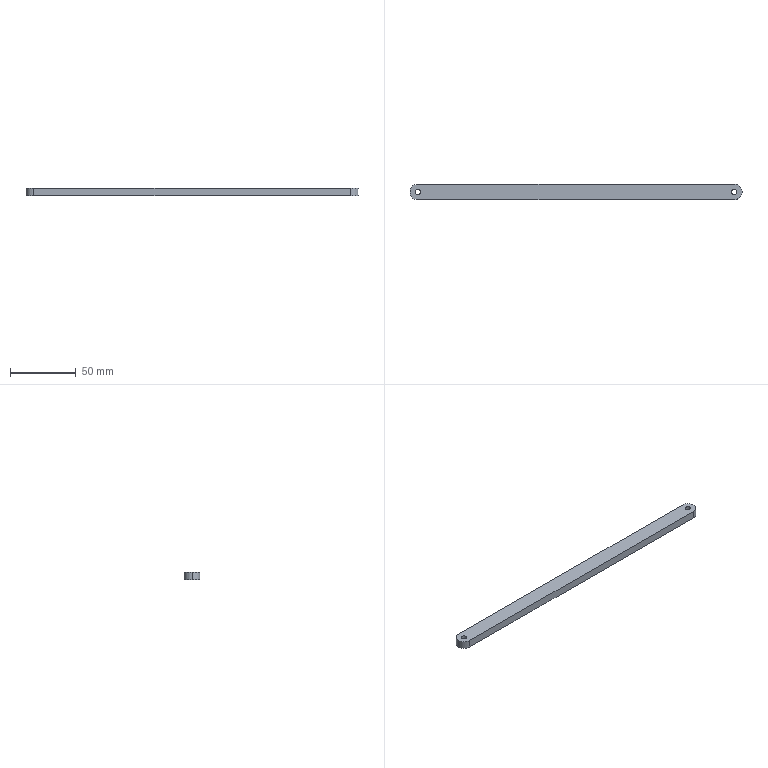Part | SolidWorks | features Extrusion 1 | 1 solid | 11 faces | box 252 x 12 x 6 mm | volume 17808 mm3 | cylinder 7 | plane 4 | commonest cylinder face diameters 4 x4 12 x3
STEP:
#1=CARTESIAN_POINT('',(118.265,1.191,6.));
#2=VERTEX_POINT('',#1);
#3=CARTESIAN_POINT('',(122.265,1.191,6.));
#4=VERTEX_POINT('',#3);
#5=CARTESIAN_POINT('',(120.265,1.191,6.));
#6=DIRECTION('',(0.,0.,1.));
#7=DIRECTION('',(1.,0.,0.));
#8=AXIS2_PLACEMENT_3D('',#5,#6,#7);
#9=CIRCLE('',#8,2.);
#10=EDGE_CURVE('',#2,#4,#9,.T.);
#11=ORIENTED_EDGE('',*,*,#10,.T.);
#12=CARTESIAN_POINT('',(122.265,1.191,0.));
#13=VERTEX_POINT('',#12);
#14=CARTESIAN_POINT('',(122.265,1.191,6.));
#15=DIRECTION('',(0.,0.,-1.));
#16=VECTOR('',#15,1000.);
#17=LINE('',#14,#16);
#18=EDGE_CURVE('',#4,#13,#17,.T.);
#19=ORIENTED_EDGE('',*,*,#18,.T.);
#20=CARTESIAN_POINT('',(118.265,1.191,0.));
#21=VERTEX_POINT('',#20);
#22=CARTESIAN_POINT('',(120.265,1.191,0.));
#23=DIRECTION('',(0.,0.,1.));
#24=DIRECTION('',(1.,0.,0.));
#25=AXIS2_PLACEMENT_3D('',#22,#23,#24);
#26=CIRCLE('',#25,2.);
#27=EDGE_CURVE('',#21,#13,#26,.T.);
#28=ORIENTED_EDGE('',*,*,#27,.F.);
#29=CARTESIAN_POINT('',(118.265,1.191,6.));
#30=DIRECTION('',(0.,0.,-1.));
#31=VECTOR('',#30,1000.);
#32=LINE('',#29,#31);
#33=EDGE_CURVE('',#2,#21,#32,.T.);
#34=ORIENTED_EDGE('',*,*,#33,.F.);
#35=EDGE_LOOP('',(#11,#19,#28,#34));
#36=FACE_OUTER_BOUND('',#35,.T.);
#37=CARTESIAN_POINT('',(120.265,1.191,6.));
#38=DIRECTION('',(0.,0.,-1.));
#39=DIRECTION('',(-1.,0.,0.));
#40=AXIS2_PLACEMENT_3D('',#37,#38,#39);
#41=CYLINDRICAL_SURFACE('',#40,2.);
#42=ADVANCED_FACE('',(#36),#41,.F.);
#43=CARTESIAN_POINT('',(-121.735,1.191,6.));
#44=VERTEX_POINT('',#43);
#45=CARTESIAN_POINT('',(-117.735,1.191,6.));
#46=VERTEX_POINT('',#45);
#47=CARTESIAN_POINT('',(-119.735,1.191,6.));
#48=DIRECTION('',(0.,0.,1.));
#49=DIRECTION('',(1.,0.,0.));
#50=AXIS2_PLACEMENT_3D('',#47,#48,#49);
#51=CIRCLE('',#50,2.);
#52=EDGE_CURVE('',#44,#46,#51,.T.);
#53=ORIENTED_EDGE('',*,*,#52,.T.);
#54=CARTESIAN_POINT('',(-117.735,1.191,0.));
#55=VERTEX_POINT('',#54);
#56=CARTESIAN_POINT('',(-117.735,1.191,6.));
#57=DIRECTION('',(0.,0.,-1.));
#58=VECTOR('',#57,1000.);
#59=LINE('',#56,#58);
#60=EDGE_CURVE('',#46,#55,#59,.T.);
#61=ORIENTED_EDGE('',*,*,#60,.T.);
#62=CARTESIAN_POINT('',(-121.735,1.191,0.));
#63=VERTEX_POINT('',#62);
#64=CARTESIAN_POINT('',(-119.735,1.191,0.));
#65=DIRECTION('',(0.,0.,1.));
#66=DIRECTION('',(1.,0.,0.));
#67=AXIS2_PLACEMENT_3D('',#64,#65,#66);
#68=CIRCLE('',#67,2.);
#69=EDGE_CURVE('',#63,#55,#68,.T.);
#70=ORIENTED_EDGE('',*,*,#69,.F.);
#71=CARTESIAN_POINT('',(-121.735,1.191,6.));
#72=DIRECTION('',(0.,0.,-1.));
#73=VECTOR('',#72,1000.);
#74=LINE('',#71,#73);
#75=EDGE_CURVE('',#44,#63,#74,.T.);
#76=ORIENTED_EDGE('',*,*,#75,.F.);
#77=EDGE_LOOP('',(#53,#61,#70,#76));
#78=FACE_OUTER_BOUND('',#77,.T.);
#79=CARTESIAN_POINT('',(-119.735,1.191,6.));
#80=DIRECTION('',(0.,0.,-1.));
#81=DIRECTION('',(-1.,0.,0.));
#82=AXIS2_PLACEMENT_3D('',#79,#80,#81);
#83=CYLINDRICAL_SURFACE('',#82,2.);
#84=ADVANCED_FACE('',(#78),#83,.F.);
#85=CARTESIAN_POINT('',(-125.735,1.191,6.));
#86=VERTEX_POINT('',#85);
#87=CARTESIAN_POINT('',(-119.735,-4.809,6.));
#88=VERTEX_POINT('',#87);
#89=CARTESIAN_POINT('',(-119.735,1.191,6.));
#90=DIRECTION('',(0.,0.,1.));
#91=DIRECTION('',(1.,0.,0.));
#92=AXIS2_PLACEMENT_3D('',#89,#90,#91);
#93=CIRCLE('',#92,6.);
#94=EDGE_CURVE('',#86,#88,#93,.T.);
#95=ORIENTED_EDGE('',*,*,#94,.F.);
#96=CARTESIAN_POINT('',(-125.735,1.191,0.));
#97=VERTEX_POINT('',#96);
#98=CARTESIAN_POINT('',(-125.735,1.191,6.));
#99=DIRECTION('',(0.,0.,-1.));
#100=VECTOR('',#99,1000.);
#101=LINE('',#98,#100);
#102=EDGE_CURVE('',#86,#97,#101,.T.);
#103=ORIENTED_EDGE('',*,*,#102,.T.);
#104=CARTESIAN_POINT('',(-119.735,-4.809,0.));
#105=VERTEX_POINT('',#104);
#106=CARTESIAN_POINT('',(-119.735,1.191,0.));
#107=DIRECTION('',(0.,0.,1.));
#108=DIRECTION('',(1.,0.,0.));
#109=AXIS2_PLACEMENT_3D('',#106,#107,#108);
#110=CIRCLE('',#109,6.);
#111=EDGE_CURVE('',#97,#105,#110,.T.);
#112=ORIENTED_EDGE('',*,*,#111,.T.);
#113=CARTESIAN_POINT('',(-119.735,-4.809,6.));
#114=DIRECTION('',(0.,0.,-1.));
#115=VECTOR('',#114,1000.);
#116=LINE('',#113,#115);
#117=EDGE_CURVE('',#88,#105,#116,.T.);
#118=ORIENTED_EDGE('',*,*,#117,.F.);
#119=EDGE_LOOP('',(#95,#103,#112,#118));
#120=FACE_OUTER_BOUND('',#119,.T.);
#121=CARTESIAN_POINT('',(-119.735,1.191,6.));
#122=DIRECTION('',(0.,0.,-1.));
#123=DIRECTION('',(-1.,0.,0.));
#124=AXIS2_PLACEMENT_3D('',#121,#122,#123);
#125=CYLINDRICAL_SURFACE('',#124,6.);
#126=ADVANCED_FACE('',(#120),#125,.T.);
#127=ORIENTED_EDGE('',*,*,#52,.F.);
#128=CARTESIAN_POINT('',(-119.735,1.191,6.));
#129=DIRECTION('',(0.,0.,1.));
#130=DIRECTION('',(1.,0.,0.));
#131=AXIS2_PLACEMENT_3D('',#128,#129,#130);
#132=CIRCLE('',#131,2.);
#133=EDGE_CURVE('',#46,#44,#132,.T.);
#134=ORIENTED_EDGE('',*,*,#133,.F.);
#135=EDGE_LOOP('',(#127,#134));
#136=FACE_BOUND('',#135,.T.);
#137=CARTESIAN_POINT('',(-119.735,7.191,6.));
#138=VERTEX_POINT('',#137);
#139=CARTESIAN_POINT('',(-119.735,1.191,6.));
#140=DIRECTION('',(0.,0.,1.));
#141=DIRECTION('',(1.,0.,0.));
#142=AXIS2_PLACEMENT_3D('',#139,#140,#141);
#143=CIRCLE('',#142,6.);
#144=EDGE_CURVE('',#138,#86,#143,.T.);
#145=ORIENTED_EDGE('',*,*,#144,.T.);
#146=ORIENTED_EDGE('',*,*,#94,.T.);
#147=CARTESIAN_POINT('',(120.265,-4.809,6.));
#148=VERTEX_POINT('',#147);
#149=CARTESIAN_POINT('',(-119.735,-4.809,6.));
#150=DIRECTION('',(1.,0.,0.));
#151=VECTOR('',#150,1000.);
#152=LINE('',#149,#151);
#153=EDGE_CURVE('',#88,#148,#152,.T.);
#154=ORIENTED_EDGE('',*,*,#153,.T.);
#155=CARTESIAN_POINT('',(120.265,7.191,6.));
#156=VERTEX_POINT('',#155);
#157=CARTESIAN_POINT('',(120.265,1.191,6.));
#158=DIRECTION('',(0.,0.,1.));
#159=DIRECTION('',(1.,0.,0.));
#160=AXIS2_PLACEMENT_3D('',#157,#158,#159);
#161=CIRCLE('',#160,6.);
#162=EDGE_CURVE('',#148,#156,#161,.T.);
#163=ORIENTED_EDGE('',*,*,#162,.T.);
#164=CARTESIAN_POINT('',(-119.735,7.191,6.));
#165=DIRECTION('',(-1.,0.,0.));
#166=VECTOR('',#165,1000.);
#167=LINE('',#164,#166);
#168=EDGE_CURVE('',#156,#138,#167,.T.);
#169=ORIENTED_EDGE('',*,*,#168,.T.);
#170=EDGE_LOOP('',(#145,#146,#154,#163,#169));
#171=FACE_OUTER_BOUND('',#170,.T.);
#172=ORIENTED_EDGE('',*,*,#10,.F.);
#173=CARTESIAN_POINT('',(120.265,1.191,6.));
#174=DIRECTION('',(0.,0.,1.));
#175=DIRECTION('',(1.,0.,0.));
#176=AXIS2_PLACEMENT_3D('',#173,#174,#175);
#177=CIRCLE('',#176,2.);
#178=EDGE_CURVE('',#4,#2,#177,.T.);
#179=ORIENTED_EDGE('',*,*,#178,.F.);
#180=EDGE_LOOP('',(#172,#179));
#181=FACE_BOUND('',#180,.T.);
#182=CARTESIAN_POINT('',(-119.735,1.191,6.));
#183=DIRECTION('',(0.,0.,1.));
#184=DIRECTION('',(1.,0.,0.));
#185=AXIS2_PLACEMENT_3D('',#182,#183,#184);
#186=PLANE('',#185);
#187=ADVANCED_FACE('',(#136,#171,#181),#186,.T.);
#188=CARTESIAN_POINT('',(-119.735,7.191,0.));
#189=VERTEX_POINT('',#188);
#190=CARTESIAN_POINT('',(-119.735,1.191,0.));
#191=DIRECTION('',(0.,0.,1.));
#192=DIRECTION('',(1.,0.,0.));
#193=AXIS2_PLACEMENT_3D('',#190,#191,#192);
#194=CIRCLE('',#193,6.);
#195=EDGE_CURVE('',#189,#97,#194,.T.);
#196=ORIENTED_EDGE('',*,*,#195,.F.);
#197=CARTESIAN_POINT('',(120.265,7.191,0.));
#198=VERTEX_POINT('',#197);
#199=CARTESIAN_POINT('',(-119.735,7.191,0.));
#200=DIRECTION('',(-1.,0.,0.));
#201=VECTOR('',#200,1000.);
#202=LINE('',#199,#201);
#203=EDGE_CURVE('',#198,#189,#202,.T.);
#204=ORIENTED_EDGE('',*,*,#203,.F.);
#205=CARTESIAN_POINT('',(120.265,-4.809,0.));
#206=VERTEX_POINT('',#205);
#207=CARTESIAN_POINT('',(120.265,1.191,0.));
#208=DIRECTION('',(0.,0.,1.));
#209=DIRECTION('',(1.,0.,0.));
#210=AXIS2_PLACEMENT_3D('',#207,#208,#209);
#211=CIRCLE('',#210,6.);
#212=EDGE_CURVE('',#206,#198,#211,.T.);
#213=ORIENTED_EDGE('',*,*,#212,.F.);
#214=CARTESIAN_POINT('',(-119.735,-4.809,0.));
#215=DIRECTION('',(1.,0.,0.));
#216=VECTOR('',#215,1000.);
#217=LINE('',#214,#216);
#218=EDGE_CURVE('',#105,#206,#217,.T.);
#219=ORIENTED_EDGE('',*,*,#218,.F.);
#220=ORIENTED_EDGE('',*,*,#111,.F.);
#221=EDGE_LOOP('',(#196,#204,#213,#219,#220));
#222=FACE_OUTER_BOUND('',#221,.T.);
#223=ORIENTED_EDGE('',*,*,#69,.T.);
#224=CARTESIAN_POINT('',(-119.735,1.191,0.));
#225=DIRECTION('',(0.,0.,1.));
#226=DIRECTION('',(1.,0.,0.));
#227=AXIS2_PLACEMENT_3D('',#224,#225,#226);
#228=CIRCLE('',#227,2.);
#229=EDGE_CURVE('',#55,#63,#228,.T.);
#230=ORIENTED_EDGE('',*,*,#229,.T.);
#231=EDGE_LOOP('',(#223,#230));
#232=FACE_BOUND('',#231,.T.);
#233=ORIENTED_EDGE('',*,*,#27,.T.);
#234=CARTESIAN_POINT('',(120.265,1.191,0.));
#235=DIRECTION('',(0.,0.,1.));
#236=DIRECTION('',(1.,0.,0.));
#237=AXIS2_PLACEMENT_3D('',#234,#235,#236);
#238=CIRCLE('',#237,2.);
#239=EDGE_CURVE('',#13,#21,#238,.T.);
#240=ORIENTED_EDGE('',*,*,#239,.T.);
#241=EDGE_LOOP('',(#233,#240));
#242=FACE_BOUND('',#241,.T.);
#243=CARTESIAN_POINT('',(-119.735,1.191,0.));
#244=DIRECTION('',(0.,0.,1.));
#245=DIRECTION('',(1.,0.,0.));
#246=AXIS2_PLACEMENT_3D('',#243,#244,#245);
#247=PLANE('',#246);
#248=ADVANCED_FACE('',(#222,#232,#242),#247,.F.);
#249=ORIENTED_EDGE('',*,*,#102,.F.);
#250=ORIENTED_EDGE('',*,*,#144,.F.);
#251=CARTESIAN_POINT('',(-119.735,7.191,6.));
#252=DIRECTION('',(0.,0.,-1.));
#253=VECTOR('',#252,1000.);
#254=LINE('',#251,#253);
#255=EDGE_CURVE('',#138,#189,#254,.T.);
#256=ORIENTED_EDGE('',*,*,#255,.T.);
#257=ORIENTED_EDGE('',*,*,#195,.T.);
#258=EDGE_LOOP('',(#249,#250,#256,#257));
#259=FACE_OUTER_BOUND('',#258,.T.);
#260=CARTESIAN_POINT('',(-119.735,1.191,6.));
#261=DIRECTION('',(0.,0.,-1.));
#262=DIRECTION('',(-1.,0.,0.));
#263=AXIS2_PLACEMENT_3D('',#260,#261,#262);
#264=CYLINDRICAL_SURFACE('',#263,6.);
#265=ADVANCED_FACE('',(#259),#264,.T.);
#266=ORIENTED_EDGE('',*,*,#218,.T.);
#267=CARTESIAN_POINT('',(120.265,-4.809,6.));
#268=DIRECTION('',(0.,0.,-1.));
#269=VECTOR('',#268,1000.);
#270=LINE('',#267,#269);
#271=EDGE_CURVE('',#148,#206,#270,.T.);
#272=ORIENTED_EDGE('',*,*,#271,.F.);
#273=ORIENTED_EDGE('',*,*,#153,.F.);
#274=ORIENTED_EDGE('',*,*,#117,.T.);
#275=EDGE_LOOP('',(#266,#272,#273,#274));
#276=FACE_OUTER_BOUND('',#275,.T.);
#277=CARTESIAN_POINT('',(-119.735,-4.809,6.));
#278=DIRECTION('',(0.,1.,0.));
#279=DIRECTION('',(0.,0.,1.));
#280=AXIS2_PLACEMENT_3D('',#277,#278,#279);
#281=PLANE('',#280);
#282=ADVANCED_FACE('',(#276),#281,.F.);
#283=ORIENTED_EDGE('',*,*,#212,.T.);
#284=CARTESIAN_POINT('',(120.265,7.191,6.));
#285=DIRECTION('',(0.,0.,-1.));
#286=VECTOR('',#285,1000.);
#287=LINE('',#284,#286);
#288=EDGE_CURVE('',#156,#198,#287,.T.);
#289=ORIENTED_EDGE('',*,*,#288,.F.);
#290=ORIENTED_EDGE('',*,*,#162,.F.);
#291=ORIENTED_EDGE('',*,*,#271,.T.);
#292=EDGE_LOOP('',(#283,#289,#290,#291));
#293=FACE_OUTER_BOUND('',#292,.T.);
#294=CARTESIAN_POINT('',(120.265,1.191,6.));
#295=DIRECTION('',(0.,0.,-1.));
#296=DIRECTION('',(-1.,0.,0.));
#297=AXIS2_PLACEMENT_3D('',#294,#295,#296);
#298=CYLINDRICAL_SURFACE('',#297,6.);
#299=ADVANCED_FACE('',(#293),#298,.T.);
#300=ORIENTED_EDGE('',*,*,#203,.T.);
#301=ORIENTED_EDGE('',*,*,#255,.F.);
#302=ORIENTED_EDGE('',*,*,#168,.F.);
#303=ORIENTED_EDGE('',*,*,#288,.T.);
#304=EDGE_LOOP('',(#300,#301,#302,#303));
#305=FACE_OUTER_BOUND('',#304,.T.);
#306=CARTESIAN_POINT('',(-119.735,7.191,6.));
#307=DIRECTION('',(0.,-1.,0.));
#308=DIRECTION('',(0.,0.,-1.));
#309=AXIS2_PLACEMENT_3D('',#306,#307,#308);
#310=PLANE('',#309);
#311=ADVANCED_FACE('',(#305),#310,.F.);
#312=ORIENTED_EDGE('',*,*,#60,.F.);
#313=ORIENTED_EDGE('',*,*,#133,.T.);
#314=ORIENTED_EDGE('',*,*,#75,.T.);
#315=ORIENTED_EDGE('',*,*,#229,.F.);
#316=EDGE_LOOP('',(#312,#313,#314,#315));
#317=FACE_OUTER_BOUND('',#316,.T.);
#318=CARTESIAN_POINT('',(-119.735,1.191,6.));
#319=DIRECTION('',(0.,0.,-1.));
#320=DIRECTION('',(-1.,0.,0.));
#321=AXIS2_PLACEMENT_3D('',#318,#319,#320);
#322=CYLINDRICAL_SURFACE('',#321,2.);
#323=ADVANCED_FACE('',(#317),#322,.F.);
#324=ORIENTED_EDGE('',*,*,#18,.F.);
#325=ORIENTED_EDGE('',*,*,#178,.T.);
#326=ORIENTED_EDGE('',*,*,#33,.T.);
#327=ORIENTED_EDGE('',*,*,#239,.F.);
#328=EDGE_LOOP('',(#324,#325,#326,#327));
#329=FACE_OUTER_BOUND('',#328,.T.);
#330=CARTESIAN_POINT('',(120.265,1.191,6.));
#331=DIRECTION('',(0.,0.,-1.));
#332=DIRECTION('',(-1.,0.,0.));
#333=AXIS2_PLACEMENT_3D('',#330,#331,#332);
#334=CYLINDRICAL_SURFACE('',#333,2.);
#335=ADVANCED_FACE('',(#329),#334,.F.);
#336=CLOSED_SHELL('',(#42,#84,#126,#187,#248,#265,#282,#299,#311,#323,#335));
#337=MANIFOLD_SOLID_BREP('',#336);
#338=CARTESIAN_POINT('',(0.,0.,0.));
#339=DIRECTION('',(0.,0.,1.));
#340=DIRECTION('',(1.,0.,0.));
#341=AXIS2_PLACEMENT_3D('',#338,#339,#340);
#342=(LENGTH_UNIT()NAMED_UNIT(*)SI_UNIT(.MILLI.,.METRE.));
#343=UNCERTAINTY_MEASURE_WITH_UNIT(LENGTH_MEASURE(0.00001),#342,'','');
#344=(NAMED_UNIT(*)PLANE_ANGLE_UNIT()SI_UNIT($,.RADIAN.));
#345=(NAMED_UNIT(*)SI_UNIT($,.STERADIAN.)SOLID_ANGLE_UNIT());
#346=(GEOMETRIC_REPRESENTATION_CONTEXT(3)GLOBAL_UNCERTAINTY_ASSIGNED_CONTEXT((#343))GLOBAL_UNIT_ASSIGNED_CONTEXT((#342,#344,#345))REPRESENTATION_CONTEXT('',''));
#347=ADVANCED_BREP_SHAPE_REPRESENTATION('',(#337,#341),#346);